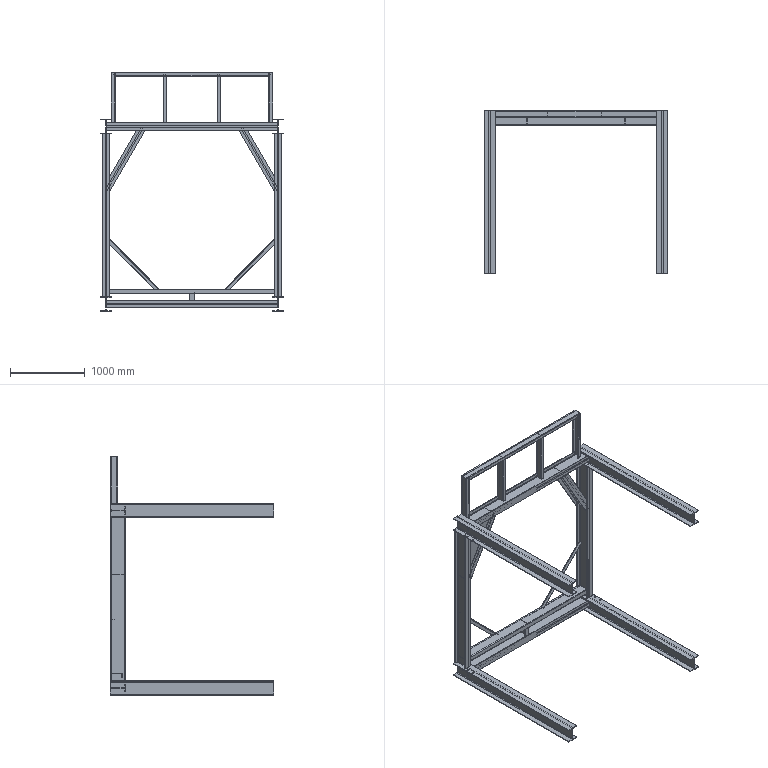Part | STEP file | 中转釜Bracket 8主体_Default<As Machined> | 21 solids | 407 faces | box 2450 x 2178 x 3187 mm | volume 74010274 mm3 | plane 315 | cylinder 92 | commonest cylinder face diameters 16 x40 19 x16 8.4 x10 17 x10 2.66 x6 10 x4